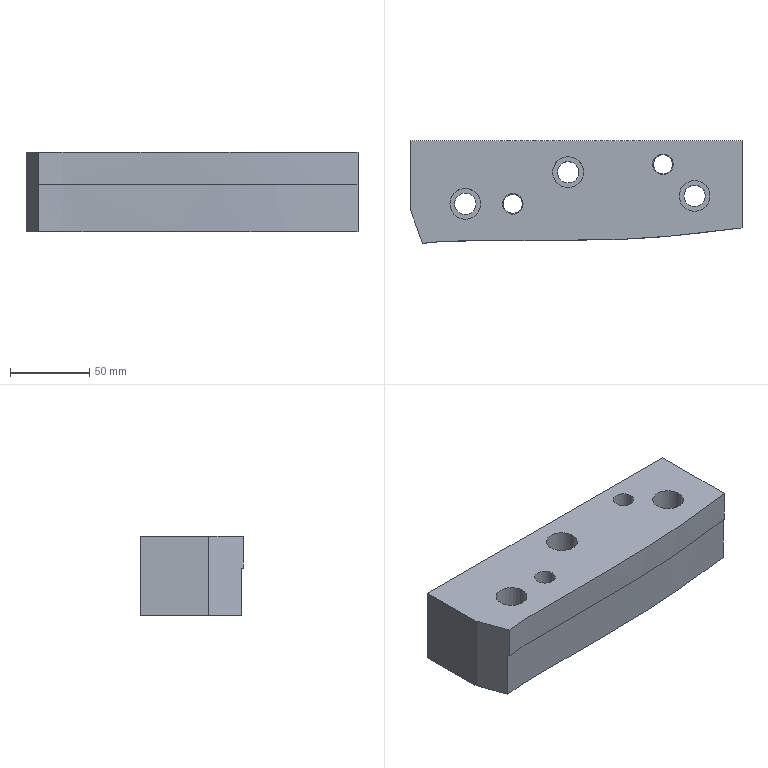Part | NX | features solid 2 | 1 solid | 24 faces | box 210 x 65.035 x 50 mm | volume 599667 mm3 | plane 12 | cylinder 10 | spline 2 | commonest cylinder face diameters 13.5 x3 19.5 x3 12 x2 13 x2
STEP:
#1=CARTESIAN_POINT('',(-107.046,-95.035,-20.));
#2=VERTEX_POINT('',#1);
#3=CARTESIAN_POINT('',(-107.046,-95.035,0.));
#4=VERTEX_POINT('',#3);
#5=CARTESIAN_POINT('',(-107.046,-95.035,-25.));
#6=DIRECTION('',(0.,0.,-1.));
#7=VECTOR('',#6,1000.);
#8=LINE('',#5,#7);
#9=EDGE_CURVE('',#2,#4,#8,.F.);
#10=ORIENTED_EDGE('',*,*,#9,.F.);
#11=CARTESIAN_POINT('',(95.,-85.269,-20.));
#12=VERTEX_POINT('',#11);
#13=CARTESIAN_POINT('',(-190.231,-121.49,-20.));
#14=CARTESIAN_POINT('',(-188.654,-121.152,-20.));
#15=CARTESIAN_POINT('',(-185.47,-120.627,-20.));
#16=CARTESIAN_POINT('',(-180.656,-120.141,-20.));
#17=CARTESIAN_POINT('',(-175.882,-119.326,-20.));
#18=CARTESIAN_POINT('',(-169.679,-117.528,-20.));
#19=CARTESIAN_POINT('',(-162.185,-114.539,-20.));
#20=CARTESIAN_POINT('',(-153.086,-111.254,-20.));
#21=CARTESIAN_POINT('',(-144.031,-107.845,-20.));
#22=CARTESIAN_POINT('',(-136.465,-105.061,-20.));
#23=CARTESIAN_POINT('',(-130.418,-102.814,-20.));
#24=CARTESIAN_POINT('',(-125.812,-101.329,-20.));
#25=CARTESIAN_POINT('',(-121.306,-99.566,-20.));
#26=CARTESIAN_POINT('',(-116.876,-97.626,-20.));
#27=CARTESIAN_POINT('',(-112.335,-95.923,-20.));
#28=CARTESIAN_POINT('',(-107.564,-95.05,-20.));
#29=CARTESIAN_POINT('',(-102.756,-94.525,-20.));
#30=CARTESIAN_POINT('',(-96.349,-93.771,-20.));
#31=CARTESIAN_POINT('',(-89.902,-93.468,-20.));
#32=CARTESIAN_POINT('',(-83.452,-93.448,-20.));
#33=CARTESIAN_POINT('',(-77.002,-93.469,-20.));
#34=CARTESIAN_POINT('',(-68.939,-93.411,-20.));
#35=CARTESIAN_POINT('',(-56.04,-93.3,-20.));
#36=CARTESIAN_POINT('',(-33.465,-93.184,-20.));
#37=CARTESIAN_POINT('',(-7.666,-93.074,-20.));
#38=CARTESIAN_POINT('',(14.907,-92.653,-20.));
#39=CARTESIAN_POINT('',(27.794,-92.068,-20.));
#40=CARTESIAN_POINT('',(40.668,-91.245,-20.));
#41=CARTESIAN_POINT('',(51.917,-90.291,-20.));
#42=CARTESIAN_POINT('',(61.528,-89.174,-20.));
#43=CARTESIAN_POINT('',(67.939,-88.466,-20.));
#44=CARTESIAN_POINT('',(79.125,-86.95,-20.));
#45=CARTESIAN_POINT('',(95.161,-85.253,-20.));
#46=CARTESIAN_POINT('',(114.404,-83.21,-20.));
#47=CARTESIAN_POINT('',(133.568,-80.524,-20.));
#48=CARTESIAN_POINT('',(152.734,-77.861,-20.));
#49=CARTESIAN_POINT('',(171.916,-75.326,-20.));
#50=CARTESIAN_POINT('',(191.055,-72.413,-20.));
#51=CARTESIAN_POINT('',(207.17,-71.468,-20.));
#52=CARTESIAN_POINT('',(219.951,-69.697,-20.));
#53=CARTESIAN_POINT('',(232.724,-67.899,-20.));
#54=CARTESIAN_POINT('',(248.708,-65.766,-20.));
#55=CARTESIAN_POINT('',(267.87,-63.074,-20.));
#56=CARTESIAN_POINT('',(287.038,-60.44,-20.));
#57=CARTESIAN_POINT('',(301.448,-58.682,-20.));
#58=CARTESIAN_POINT('',(310.976,-56.987,-20.));
#59=CARTESIAN_POINT('',(314.916,-56.135,-20.));
#60=CARTESIAN_POINT('',(318.052,-55.382,-20.));
#61=CARTESIAN_POINT('',(320.39,-54.76,-20.));
#62=CARTESIAN_POINT('',(322.686,-53.981,-20.));
#63=CARTESIAN_POINT('',(325.595,-52.578,-20.));
#64=CARTESIAN_POINT('',(328.769,-50.098,-20.));
#65=CARTESIAN_POINT('',(332.247,-46.69,-20.));
#66=CARTESIAN_POINT('',(335.795,-43.406,-20.));
#67=CARTESIAN_POINT('',(343.661,-37.758,-20.));
#68=CARTESIAN_POINT('',(355.164,-28.914,-20.));
#69=CARTESIAN_POINT('',(370.422,-17.018,-20.));
#70=CARTESIAN_POINT('',(383.264,-7.249,-20.));
#71=CARTESIAN_POINT('',(392.416,-0.6713,-20.));
#72=CARTESIAN_POINT('',(396.953,2.733,-20.));
#73=CARTESIAN_POINT('',(398.886,5.372,-20.));
#74=CARTESIAN_POINT('',(399.725,7.654,-20.));
#75=CARTESIAN_POINT('',(399.76,10.078,-20.));
#76=CARTESIAN_POINT('',(399.483,13.317,-20.));
#77=CARTESIAN_POINT('',(399.712,17.34,-20.));
#78=CARTESIAN_POINT('',(399.612,22.179,-20.));
#79=CARTESIAN_POINT('',(399.633,31.854,-20.));
#80=CARTESIAN_POINT('',(399.593,46.366,-20.));
#81=CARTESIAN_POINT('',(399.637,62.491,-20.));
#82=CARTESIAN_POINT('',(399.588,73.779,-20.));
#83=CARTESIAN_POINT('',(399.652,79.422,-20.));
#84=CARTESIAN_POINT('',(399.59,82.647,-20.));
#85=CARTESIAN_POINT('',(399.564,85.065,-20.));
#86=CARTESIAN_POINT('',(399.725,87.486,-20.));
#87=CARTESIAN_POINT('',(399.756,89.902,-20.));
#88=CARTESIAN_POINT('',(399.247,92.301,-20.));
#89=CARTESIAN_POINT('',(397.362,95.008,-20.));
#90=CARTESIAN_POINT('',(393.635,96.774,-20.));
#91=CARTESIAN_POINT('',(389.279,98.826,-20.));
#92=CARTESIAN_POINT('',(384.732,100.498,-20.));
#93=CARTESIAN_POINT('',(378.765,102.95,-20.));
#94=CARTESIAN_POINT('',(362.589,110.229,-20.));
#95=CARTESIAN_POINT('',(344.928,118.135,-20.));
#96=CARTESIAN_POINT('',(327.281,126.072,-20.));
#97=CARTESIAN_POINT('',(319.932,129.381,-20.));
#98=CARTESIAN_POINT('',(314.075,132.102,-20.));
#99=CARTESIAN_POINT('',(309.387,133.376,-20.));
#100=CARTESIAN_POINT('',(304.547,133.785,-20.));
#101=CARTESIAN_POINT('',(299.716,133.401,-20.));
#102=CARTESIAN_POINT('',(294.929,132.704,-20.));
#103=CARTESIAN_POINT('',(288.543,131.8,-20.));
#104=CARTESIAN_POINT('',(277.364,130.241,-20.));
#105=CARTESIAN_POINT('',(242.2,125.552,-20.));
#106=CARTESIAN_POINT('',(184.637,118.048,-20.));
#107=CARTESIAN_POINT('',(120.701,109.541,-20.));
#108=CARTESIAN_POINT('',(69.531,102.902,-20.));
#109=CARTESIAN_POINT('',(40.777,98.94,-20.));
#110=CARTESIAN_POINT('',(21.566,96.615,-20.));
#111=CARTESIAN_POINT('',(8.743,95.212,-20.));
#112=CARTESIAN_POINT('',(-7.301,93.575,-20.));
#113=CARTESIAN_POINT('',(-26.625,92.505,-20.));
#114=CARTESIAN_POINT('',(-45.971,92.017,-20.));
#115=CARTESIAN_POINT('',(-62.09,91.675,-20.));
#116=CARTESIAN_POINT('',(-74.987,91.256,-20.));
#117=CARTESIAN_POINT('',(-84.664,91.165,-20.));
#118=CARTESIAN_POINT('',(-94.319,91.781,-20.));
#119=CARTESIAN_POINT('',(-103.929,92.966,-20.));
#120=CARTESIAN_POINT('',(-113.495,94.403,-20.));
#121=CARTESIAN_POINT('',(-119.856,95.492,-20.));
#122=CARTESIAN_POINT('',(-122.997,96.222,-20.));
#123=B_SPLINE_CURVE_WITH_KNOTS('',3,(#13,#14,#15,#16,#17,#18,#19,#20,#21,#22,#23,#24,#25,#26,#27,#28,#29,#30,#31,#32,#33,#34,#35,#36,#37,#38,#39,#40,#41,#42,#43,#44,#45,#46,#47,#48,#49,#50,#51,#52,#53,#54,#55,#56,#57,#58,#59,#60,#61,#62,#63,#64,#65,#66,#67,#68,#69,#70,#71,#72,#73,#74,#75,#76,#77,#78,#79,#80,#81,#82,#83,#84,#85,#86,#87,#88,#89,#90,#91,#92,#93,#94,#95,#96,#97,#98,#99,#100,#101,#102,#103,#104,#105,#106,#107,#108,#109,#110,#111,#112,#113,#114,#115,#116,#117,#118,#119,#120,#121,#122),.UNSPECIFIED.,.F.,.F.,(4,1,1,1,1,1,1,1,1,1,1,1,1,1,1,1,1,1,1,1,1,1,1,1,1,1,1,1,1,1,1,1,1,1,1,1,1,1,1,1,1,1,1,1,1,1,1,1,1,1,1,1,1,1,1,1,1,1,1,1,1,1,1,1,1,1,1,1,1,1,1,1,1,1,1,1,1,1,1,1,1,1,1,1,1,1,1,1,1,1,1,1,1,1,1,1,1,1,1,1,1,1,1,1,1,1,1,4),(0.4704,0.4724,0.4745,0.4766,0.4786,0.4828,0.4869,0.491,0.4952,0.4972,0.4993,0.5014,0.5035,0.5055,0.5076,0.5097,0.5117,0.5159,0.5179,0.52,0.5241,0.5283,0.5366,0.5531,0.5614,0.5655,0.5697,0.5779,0.58,0.5821,0.5862,0.5945,0.6028,0.611,0.6193,0.6276,0.6359,0.6441,0.6483,0.6524,0.6607,0.669,0.6772,0.6855,0.6876,0.6897,0.6907,0.6917,0.6928,0.6938,0.6959,0.6979,0.7,0.7021,0.7103,0.7186,0.7269,0.731,0.7331,0.7341,0.7352,0.7362,0.7372,0.7393,0.7414,0.7435,0.7517,0.76,0.7641,0.7662,0.7672,0.7683,0.7693,0.7703,0.7714,0.7724,0.7745,0.7766,0.7786,0.7807,0.7848,0.8014,0.8055,0.8097,0.8117,0.8138,0.8159,0.8179,0.82,0.8221,0.8262,0.8345,0.8676,0.9007,0.9172,0.9338,0.9379,0.9421,0.9503,0.9586,0.9669,0.9752,0.9793,0.9834,0.9876,0.9917,0.9959,1.),.UNSPECIFIED.);
#124=EDGE_CURVE('',#2,#12,#123,.T.);
#125=ORIENTED_EDGE('',*,*,#124,.T.);
#126=CARTESIAN_POINT('',(95.,-85.269,0.));
#127=VERTEX_POINT('',#126);
#128=CARTESIAN_POINT('',(95.,-85.269,-10.));
#129=DIRECTION('',(0.,0.,-1.));
#130=VECTOR('',#129,1000.);
#131=LINE('',#128,#130);
#132=EDGE_CURVE('',#127,#12,#131,.T.);
#133=ORIENTED_EDGE('',*,*,#132,.F.);
#134=CARTESIAN_POINT('',(95.,-85.269,0.));
#135=CARTESIAN_POINT('',(90.809,-85.713,0.));
#136=CARTESIAN_POINT('',(82.426,-86.582,0.));
#137=CARTESIAN_POINT('',(69.877,-88.217,0.));
#138=CARTESIAN_POINT('',(57.316,-89.701,0.));
#139=CARTESIAN_POINT('',(40.542,-91.326,0.));
#140=CARTESIAN_POINT('',(19.52,-92.617,0.));
#141=CARTESIAN_POINT('',(-5.792,-93.02,0.));
#142=CARTESIAN_POINT('',(-31.119,-93.19,0.));
#143=CARTESIAN_POINT('',(-52.226,-93.263,0.));
#144=CARTESIAN_POINT('',(-69.108,-93.423,0.));
#145=CARTESIAN_POINT('',(-81.772,-93.467,0.));
#146=CARTESIAN_POINT('',(-92.328,-93.446,0.));
#147=CARTESIAN_POINT('',(-100.741,-94.276,0.));
#148=CARTESIAN_POINT('',(-104.946,-94.744,0.));
#149=CARTESIAN_POINT('',(-107.046,-95.035,0.));
#150=B_SPLINE_CURVE_WITH_KNOTS('',3,(#134,#135,#136,#137,#138,#139,#140,#141,#142,#143,#144,#145,#146,#147,#148,#149),.UNSPECIFIED.,.F.,.F.,(4,1,1,1,1,1,1,1,1,1,1,1,1,4),(0.,0.01264,0.02527,0.03791,0.05054,0.07582,0.1011,0.1264,0.1516,0.1643,0.1769,0.1895,0.1959,0.2022),.UNSPECIFIED.);
#151=EDGE_CURVE('',#127,#4,#150,.T.);
#152=ORIENTED_EDGE('',*,*,#151,.T.);
#153=EDGE_LOOP('',(#10,#125,#133,#152));
#154=FACE_BOUND('',#153,.T.);
#155=CARTESIAN_POINT('',(-107.046,-95.035,0.));
#156=CARTESIAN_POINT('',(-107.046,-95.035,-20.));
#157=CARTESIAN_POINT('',(-104.956,-94.746,0.));
#158=CARTESIAN_POINT('',(-104.956,-94.746,-20.));
#159=CARTESIAN_POINT('',(-100.763,-94.279,0.));
#160=CARTESIAN_POINT('',(-100.763,-94.279,-20.));
#161=CARTESIAN_POINT('',(-92.365,-93.447,0.));
#162=CARTESIAN_POINT('',(-92.365,-93.447,-20.));
#163=CARTESIAN_POINT('',(-81.808,-93.466,0.));
#164=CARTESIAN_POINT('',(-81.808,-93.466,-20.));
#165=CARTESIAN_POINT('',(-69.155,-93.424,0.));
#166=CARTESIAN_POINT('',(-69.155,-93.424,-20.));
#167=CARTESIAN_POINT('',(-52.28,-93.263,0.));
#168=CARTESIAN_POINT('',(-52.28,-93.263,-20.));
#169=CARTESIAN_POINT('',(-31.187,-93.19,0.));
#170=CARTESIAN_POINT('',(-31.187,-93.19,-20.));
#171=CARTESIAN_POINT('',(-5.876,-93.02,0.));
#172=CARTESIAN_POINT('',(-5.876,-93.02,-20.));
#173=CARTESIAN_POINT('',(19.435,-92.62,0.));
#174=CARTESIAN_POINT('',(19.435,-92.62,-20.));
#175=CARTESIAN_POINT('',(40.496,-91.329,0.));
#176=CARTESIAN_POINT('',(40.496,-91.329,-20.));
#177=CARTESIAN_POINT('',(57.293,-89.704,0.));
#178=CARTESIAN_POINT('',(57.293,-89.704,-20.));
#179=CARTESIAN_POINT('',(69.862,-88.219,0.));
#180=CARTESIAN_POINT('',(69.862,-88.219,-20.));
#181=CARTESIAN_POINT('',(82.412,-86.583,0.));
#182=CARTESIAN_POINT('',(82.412,-86.583,-20.));
#183=CARTESIAN_POINT('',(90.805,-85.714,0.));
#184=CARTESIAN_POINT('',(90.805,-85.714,-20.));
#185=CARTESIAN_POINT('',(95.,-85.269,0.));
#186=CARTESIAN_POINT('',(95.,-85.269,-20.));
#187=B_SPLINE_SURFACE_WITH_KNOTS('',3,1,((#155,#156),(#157,#158),(#159,#160),(#161,#162),(#163,#164),(#165,#166),(#167,#168),(#169,#170),(#171,#172),(#173,#174),(#175,#176),(#177,#178),(#179,#180),(#181,#182),(#183,#184),(#185,#186)),.SURF_OF_LINEAR_EXTRUSION.,.F.,.F.,.F.,(4,1,1,1,1,1,1,1,1,1,1,1,1,4),(2,2),(0.5078,0.5105,0.5132,0.5186,0.5241,0.5295,0.5403,0.5511,0.5619,0.5728,0.5782,0.5836,0.589,0.5944),(0.,1.),.UNSPECIFIED.);
#188=ADVANCED_FACE('',(#154),#187,.F.);
#189=CARTESIAN_POINT('',(95.,-84.264,-20.));
#190=VERTEX_POINT('',#189);
#191=CARTESIAN_POINT('',(95.,83.097,-20.));
#192=DIRECTION('',(0.,-1.,0.));
#193=VECTOR('',#192,1000.);
#194=LINE('',#191,#193);
#195=EDGE_CURVE('',#190,#12,#194,.T.);
#196=ORIENTED_EDGE('',*,*,#195,.F.);
#197=CARTESIAN_POINT('',(95.,-84.264,-50.));
#198=VERTEX_POINT('',#197);
#199=CARTESIAN_POINT('',(95.,-84.264,-60.));
#200=DIRECTION('',(0.,0.,-1.));
#201=VECTOR('',#200,1000.);
#202=LINE('',#199,#201);
#203=EDGE_CURVE('',#198,#190,#202,.F.);
#204=ORIENTED_EDGE('',*,*,#203,.F.);
#205=CARTESIAN_POINT('',(95.,-30.,-50.));
#206=VERTEX_POINT('',#205);
#207=CARTESIAN_POINT('',(95.,35.09,-50.));
#208=DIRECTION('',(0.,1.,0.));
#209=VECTOR('',#208,1000.);
#210=LINE('',#207,#209);
#211=EDGE_CURVE('',#198,#206,#210,.T.);
#212=ORIENTED_EDGE('',*,*,#211,.T.);
#213=CARTESIAN_POINT('',(95.,-30.,0.));
#214=VERTEX_POINT('',#213);
#215=CARTESIAN_POINT('',(95.,-30.,0.));
#216=DIRECTION('',(0.,0.,-1.));
#217=VECTOR('',#216,1000.);
#218=LINE('',#215,#217);
#219=EDGE_CURVE('',#214,#206,#218,.T.);
#220=ORIENTED_EDGE('',*,*,#219,.F.);
#221=CARTESIAN_POINT('',(95.,-222.,0.));
#222=DIRECTION('',(0.,-1.,0.));
#223=VECTOR('',#222,1000.);
#224=LINE('',#221,#223);
#225=EDGE_CURVE('',#214,#127,#224,.T.);
#226=ORIENTED_EDGE('',*,*,#225,.T.);
#227=ORIENTED_EDGE('',*,*,#132,.T.);
#228=EDGE_LOOP('',(#196,#204,#212,#220,#226,#227));
#229=FACE_BOUND('',#228,.T.);
#230=CARTESIAN_POINT('',(95.,83.097,-25.));
#231=DIRECTION('',(1.,0.,0.));
#232=DIRECTION('',(0.,0.,-1.));
#233=AXIS2_PLACEMENT_3D('',#230,#231,#232);
#234=PLANE('',#233);
#235=ADVANCED_FACE('',(#229),#234,.T.);
#236=CARTESIAN_POINT('',(-115.,-73.182,-50.));
#237=VERTEX_POINT('',#236);
#238=CARTESIAN_POINT('',(-115.,-30.,-50.));
#239=VERTEX_POINT('',#238);
#240=CARTESIAN_POINT('',(-115.,35.09,-50.));
#241=DIRECTION('',(0.,1.,0.));
#242=VECTOR('',#241,1000.);
#243=LINE('',#240,#242);
#244=EDGE_CURVE('',#237,#239,#243,.T.);
#245=ORIENTED_EDGE('',*,*,#244,.F.);
#246=CARTESIAN_POINT('',(-115.,-73.182,0.));
#247=VERTEX_POINT('',#246);
#248=CARTESIAN_POINT('',(-115.,-73.182,0.));
#249=DIRECTION('',(0.,0.,1.));
#250=VECTOR('',#249,1000.);
#251=LINE('',#248,#250);
#252=EDGE_CURVE('',#237,#247,#251,.T.);
#253=ORIENTED_EDGE('',*,*,#252,.T.);
#254=CARTESIAN_POINT('',(-115.,-30.,0.));
#255=VERTEX_POINT('',#254);
#256=CARTESIAN_POINT('',(-115.,-222.,0.));
#257=DIRECTION('',(0.,-1.,0.));
#258=VECTOR('',#257,1000.);
#259=LINE('',#256,#258);
#260=EDGE_CURVE('',#255,#247,#259,.T.);
#261=ORIENTED_EDGE('',*,*,#260,.F.);
#262=CARTESIAN_POINT('',(-115.,-30.,0.));
#263=DIRECTION('',(0.,0.,1.));
#264=VECTOR('',#263,1000.);
#265=LINE('',#262,#264);
#266=EDGE_CURVE('',#239,#255,#265,.T.);
#267=ORIENTED_EDGE('',*,*,#266,.F.);
#268=EDGE_LOOP('',(#245,#253,#261,#267));
#269=FACE_BOUND('',#268,.T.);
#270=CARTESIAN_POINT('',(-115.,30.,0.));
#271=DIRECTION('',(1.,0.,0.));
#272=DIRECTION('',(0.,0.,-1.));
#273=AXIS2_PLACEMENT_3D('',#270,#271,#272);
#274=PLANE('',#273);
#275=ADVANCED_FACE('',(#269),#274,.F.);
#276=CARTESIAN_POINT('',(-56.5,-70.,0.));
#277=VERTEX_POINT('',#276);
#278=CARTESIAN_POINT('',(-50.,-70.,0.));
#279=DIRECTION('',(0.,0.,-1.));
#280=DIRECTION('',(-1.,0.,0.));
#281=AXIS2_PLACEMENT_3D('',#278,#279,#280);
#282=CIRCLE('',#281,6.5);
#283=EDGE_CURVE('',#277,#277,#282,.T.);
#284=ORIENTED_EDGE('',*,*,#283,.T.);
#285=EDGE_LOOP('',(#284));
#286=FACE_BOUND('',#285,.T.);
#287=CARTESIAN_POINT('',(38.5,-45.,0.));
#288=VERTEX_POINT('',#287);
#289=CARTESIAN_POINT('',(45.,-45.,0.));
#290=DIRECTION('',(0.,0.,-1.));
#291=DIRECTION('',(-1.,0.,0.));
#292=AXIS2_PLACEMENT_3D('',#289,#290,#291);
#293=CIRCLE('',#292,6.5);
#294=EDGE_CURVE('',#288,#288,#293,.T.);
#295=ORIENTED_EDGE('',*,*,#294,.T.);
#296=EDGE_LOOP('',(#295));
#297=FACE_BOUND('',#296,.T.);
#298=CARTESIAN_POINT('',(-89.75,-70.,0.));
#299=VERTEX_POINT('',#298);
#300=CARTESIAN_POINT('',(-80.,-70.,0.));
#301=DIRECTION('',(0.,0.,-1.));
#302=DIRECTION('',(-1.,0.,0.));
#303=AXIS2_PLACEMENT_3D('',#300,#301,#302);
#304=CIRCLE('',#303,9.75);
#305=EDGE_CURVE('',#299,#299,#304,.T.);
#306=ORIENTED_EDGE('',*,*,#305,.T.);
#307=EDGE_LOOP('',(#306));
#308=FACE_BOUND('',#307,.T.);
#309=CARTESIAN_POINT('',(-24.75,-50.,0.));
#310=VERTEX_POINT('',#309);
#311=CARTESIAN_POINT('',(-15.,-50.,0.));
#312=DIRECTION('',(0.,0.,-1.));
#313=DIRECTION('',(-1.,0.,0.));
#314=AXIS2_PLACEMENT_3D('',#311,#312,#313);
#315=CIRCLE('',#314,9.75);
#316=EDGE_CURVE('',#310,#310,#315,.T.);
#317=ORIENTED_EDGE('',*,*,#316,.T.);
#318=EDGE_LOOP('',(#317));
#319=FACE_BOUND('',#318,.T.);
#320=CARTESIAN_POINT('',(55.25,-65.,0.));
#321=VERTEX_POINT('',#320);
#322=CARTESIAN_POINT('',(65.,-65.,0.));
#323=DIRECTION('',(0.,0.,-1.));
#324=DIRECTION('',(-1.,0.,0.));
#325=AXIS2_PLACEMENT_3D('',#322,#323,#324);
#326=CIRCLE('',#325,9.75);
#327=EDGE_CURVE('',#321,#321,#326,.T.);
#328=ORIENTED_EDGE('',*,*,#327,.T.);
#329=EDGE_LOOP('',(#328));
#330=FACE_BOUND('',#329,.T.);
#331=ORIENTED_EDGE('',*,*,#260,.T.);
#332=CARTESIAN_POINT('',(-108.743,-90.374,0.));
#333=DIRECTION('',(0.342,-0.9397,0.));
#334=VECTOR('',#333,1000.);
#335=LINE('',#332,#334);
#336=EDGE_CURVE('',#247,#4,#335,.T.);
#337=ORIENTED_EDGE('',*,*,#336,.T.);
#338=ORIENTED_EDGE('',*,*,#151,.F.);
#339=ORIENTED_EDGE('',*,*,#225,.F.);
#340=CARTESIAN_POINT('',(-470.381,-30.,0.));
#341=DIRECTION('',(1.,0.,0.));
#342=VECTOR('',#341,1000.);
#343=LINE('',#340,#342);
#344=EDGE_CURVE('',#255,#214,#343,.T.);
#345=ORIENTED_EDGE('',*,*,#344,.F.);
#346=EDGE_LOOP('',(#331,#337,#338,#339,#345));
#347=FACE_BOUND('',#346,.T.);
#348=CARTESIAN_POINT('',(-470.381,-222.,0.));
#349=DIRECTION('',(0.,0.,-1.));
#350=DIRECTION('',(-1.,0.,0.));
#351=AXIS2_PLACEMENT_3D('',#348,#349,#350);
#352=PLANE('',#351);
#353=ADVANCED_FACE('',(#286,#297,#308,#319,#330,#347),#352,.F.);
#354=ORIENTED_EDGE('',*,*,#344,.T.);
#355=ORIENTED_EDGE('',*,*,#219,.T.);
#356=CARTESIAN_POINT('',(-415.478,-30.,-50.));
#357=DIRECTION('',(-1.,0.,0.));
#358=VECTOR('',#357,1000.);
#359=LINE('',#356,#358);
#360=EDGE_CURVE('',#206,#239,#359,.T.);
#361=ORIENTED_EDGE('',*,*,#360,.T.);
#362=ORIENTED_EDGE('',*,*,#266,.T.);
#363=EDGE_LOOP('',(#354,#355,#361,#362));
#364=FACE_BOUND('',#363,.T.);
#365=CARTESIAN_POINT('',(190.,-30.,0.));
#366=DIRECTION('',(0.,1.,0.));
#367=DIRECTION('',(0.,0.,1.));
#368=AXIS2_PLACEMENT_3D('',#365,#366,#367);
#369=PLANE('',#368);
#370=ADVANCED_FACE('',(#364),#369,.T.);
#371=CARTESIAN_POINT('',(-44.,-70.,-50.));
#372=VERTEX_POINT('',#371);
#373=CARTESIAN_POINT('',(-50.,-70.,-50.));
#374=DIRECTION('',(0.,0.,1.));
#375=DIRECTION('',(1.,0.,0.));
#376=AXIS2_PLACEMENT_3D('',#373,#374,#375);
#377=CIRCLE('',#376,6.);
#378=EDGE_CURVE('',#372,#372,#377,.T.);
#379=ORIENTED_EDGE('',*,*,#378,.T.);
#380=EDGE_LOOP('',(#379));
#381=FACE_BOUND('',#380,.T.);
#382=CARTESIAN_POINT('',(51.,-45.,-50.));
#383=VERTEX_POINT('',#382);
#384=CARTESIAN_POINT('',(45.,-45.,-50.));
#385=DIRECTION('',(0.,0.,1.));
#386=DIRECTION('',(1.,0.,0.));
#387=AXIS2_PLACEMENT_3D('',#384,#385,#386);
#388=CIRCLE('',#387,6.);
#389=EDGE_CURVE('',#383,#383,#388,.T.);
#390=ORIENTED_EDGE('',*,*,#389,.T.);
#391=EDGE_LOOP('',(#390));
#392=FACE_BOUND('',#391,.T.);
#393=CARTESIAN_POINT('',(-73.25,-70.,-50.));
#394=VERTEX_POINT('',#393);
#395=CARTESIAN_POINT('',(-80.,-70.,-50.));
#396=DIRECTION('',(0.,0.,1.));
#397=DIRECTION('',(1.,0.,0.));
#398=AXIS2_PLACEMENT_3D('',#395,#396,#397);
#399=CIRCLE('',#398,6.75);
#400=EDGE_CURVE('',#394,#394,#399,.T.);
#401=ORIENTED_EDGE('',*,*,#400,.T.);
#402=EDGE_LOOP('',(#401));
#403=FACE_BOUND('',#402,.T.);
#404=CARTESIAN_POINT('',(-8.25,-50.,-50.));
#405=VERTEX_POINT('',#404);
#406=CARTESIAN_POINT('',(-15.,-50.,-50.));
#407=DIRECTION('',(0.,0.,1.));
#408=DIRECTION('',(1.,0.,0.));
#409=AXIS2_PLACEMENT_3D('',#406,#407,#408);
#410=CIRCLE('',#409,6.75);
#411=EDGE_CURVE('',#405,#405,#410,.T.);
#412=ORIENTED_EDGE('',*,*,#411,.T.);
#413=EDGE_LOOP('',(#412));
#414=FACE_BOUND('',#413,.T.);
#415=CARTESIAN_POINT('',(71.75,-65.,-50.));
#416=VERTEX_POINT('',#415);
#417=CARTESIAN_POINT('',(65.,-65.,-50.));
#418=DIRECTION('',(0.,0.,1.));
#419=DIRECTION('',(1.,0.,0.));
#420=AXIS2_PLACEMENT_3D('',#417,#418,#419);
#421=CIRCLE('',#420,6.75);
#422=EDGE_CURVE('',#416,#416,#421,.T.);
#423=ORIENTED_EDGE('',*,*,#422,.T.);
#424=EDGE_LOOP('',(#423));
#425=FACE_BOUND('',#424,.T.);
#426=ORIENTED_EDGE('',*,*,#211,.F.);
#427=CARTESIAN_POINT('',(-107.396,-94.075,-50.));
#428=VERTEX_POINT('',#427);
#429=CARTESIAN_POINT('',(95.,-84.264,-50.));
#430=CARTESIAN_POINT('',(90.802,-84.709,-50.));
#431=CARTESIAN_POINT('',(82.405,-85.578,-50.));
#432=CARTESIAN_POINT('',(69.834,-87.213,-50.));
#433=CARTESIAN_POINT('',(57.253,-88.703,-50.));
#434=CARTESIAN_POINT('',(40.45,-90.33,-50.));
#435=CARTESIAN_POINT('',(19.392,-91.622,-50.));
#436=CARTESIAN_POINT('',(-5.964,-92.021,-50.));
#437=CARTESIAN_POINT('',(-31.334,-92.191,-50.));
#438=CARTESIAN_POINT('',(-52.477,-92.263,-50.));
#439=CARTESIAN_POINT('',(-69.388,-92.427,-50.));
#440=CARTESIAN_POINT('',(-82.074,-92.461,-50.));
#441=CARTESIAN_POINT('',(-92.647,-92.457,-50.));
#442=CARTESIAN_POINT('',(-101.077,-93.311,-50.));
#443=CARTESIAN_POINT('',(-105.291,-93.777,-50.));
#444=CARTESIAN_POINT('',(-107.396,-94.075,-50.));
#445=B_SPLINE_CURVE_WITH_KNOTS('',3,(#429,#430,#431,#432,#433,#434,#435,#436,#437,#438,#439,#440,#441,#442,#443,#444),.UNSPECIFIED.,.F.,.F.,(4,1,1,1,1,1,1,1,1,1,1,1,1,4),(0.,0.01266,0.02532,0.03797,0.05063,0.07595,0.1013,0.1266,0.1519,0.1645,0.1772,0.1899,0.1962,0.2025),.UNSPECIFIED.);
#446=EDGE_CURVE('',#198,#428,#445,.T.);
#447=ORIENTED_EDGE('',*,*,#446,.T.);
#448=CARTESIAN_POINT('',(-184.947,118.996,-50.));
#449=DIRECTION('',(-0.342,0.9397,0.));
#450=VECTOR('',#449,1000.);
#451=LINE('',#448,#450);
#452=EDGE_CURVE('',#428,#237,#451,.T.);
#453=ORIENTED_EDGE('',*,*,#452,.T.);
#454=ORIENTED_EDGE('',*,*,#244,.T.);
#455=ORIENTED_EDGE('',*,*,#360,.F.);
#456=EDGE_LOOP('',(#426,#447,#453,#454,#455));
#457=FACE_BOUND('',#456,.T.);
#458=CARTESIAN_POINT('',(-415.478,35.09,-50.));
#459=DIRECTION('',(0.,0.,1.));
#460=DIRECTION('',(1.,0.,0.));
#461=AXIS2_PLACEMENT_3D('',#458,#459,#460);
#462=PLANE('',#461);
#463=ADVANCED_FACE('',(#381,#392,#403,#414,#425,#457),#462,.F.);
#464=CARTESIAN_POINT('',(58.25,-65.,-15.));
#465=VERTEX_POINT('',#464);
#466=CARTESIAN_POINT('',(65.,-65.,-15.));
#467=DIRECTION('',(0.,0.,-1.));
#468=DIRECTION('',(-1.,0.,0.));
#469=AXIS2_PLACEMENT_3D('',#466,#467,#468);
#470=CIRCLE('',#469,6.75);
#471=EDGE_CURVE('',#465,#465,#470,.T.);
#472=ORIENTED_EDGE('',*,*,#471,.F.);
#473=EDGE_LOOP('',(#472));
#474=FACE_BOUND('',#473,.T.);
#475=ORIENTED_EDGE('',*,*,#422,.F.);
#476=EDGE_LOOP('',(#475));
#477=FACE_BOUND('',#476,.T.);
#478=CARTESIAN_POINT('',(65.,-65.,-100.));
#479=DIRECTION('',(0.,0.,-1.));
#480=DIRECTION('',(-1.,0.,0.));
#481=AXIS2_PLACEMENT_3D('',#478,#479,#480);
#482=CYLINDRICAL_SURFACE('',#481,6.75);
#483=ADVANCED_FACE('',(#474,#477),#482,.F.);
#484=ORIENTED_EDGE('',*,*,#471,.T.);
#485=EDGE_LOOP('',(#484));
#486=FACE_BOUND('',#485,.T.);
#487=CARTESIAN_POINT('',(55.25,-65.,-15.));
#488=VERTEX_POINT('',#487);
#489=CARTESIAN_POINT('',(65.,-65.,-15.));
#490=DIRECTION('',(0.,0.,-1.));
#491=DIRECTION('',(-1.,0.,0.));
#492=AXIS2_PLACEMENT_3D('',#489,#490,#491);
#493=CIRCLE('',#492,9.75);
#494=EDGE_CURVE('',#488,#488,#493,.T.);
#495=ORIENTED_EDGE('',*,*,#494,.F.);
#496=EDGE_LOOP('',(#495));
#497=FACE_BOUND('',#496,.T.);
#498=CARTESIAN_POINT('',(65.,-65.,-15.));
#499=DIRECTION('',(0.,0.,-1.));
#500=DIRECTION('',(-1.,0.,0.));
#501=AXIS2_PLACEMENT_3D('',#498,#499,#500);
#502=PLANE('',#501);
#503=ADVANCED_FACE('',(#486,#497),#502,.F.);
#504=ORIENTED_EDGE('',*,*,#494,.T.);
#505=EDGE_LOOP('',(#504));
#506=FACE_BOUND('',#505,.T.);
#507=ORIENTED_EDGE('',*,*,#327,.F.);
#508=EDGE_LOOP('',(#507));
#509=FACE_BOUND('',#508,.T.);
#510=CARTESIAN_POINT('',(65.,-65.,0.));
#511=DIRECTION('',(0.,0.,-1.));
#512=DIRECTION('',(-1.,0.,0.));
#513=AXIS2_PLACEMENT_3D('',#510,#511,#512);
#514=CYLINDRICAL_SURFACE('',#513,9.75);
#515=ADVANCED_FACE('',(#506,#509),#514,.F.);
#516=CARTESIAN_POINT('',(-21.75,-50.,-15.));
#517=VERTEX_POINT('',#516);
#518=CARTESIAN_POINT('',(-15.,-50.,-15.));
#519=DIRECTION('',(0.,0.,-1.));
#520=DIRECTION('',(-1.,0.,0.));
#521=AXIS2_PLACEMENT_3D('',#518,#519,#520);
#522=CIRCLE('',#521,6.75);
#523=EDGE_CURVE('',#517,#517,#522,.T.);
#524=ORIENTED_EDGE('',*,*,#523,.F.);
#525=EDGE_LOOP('',(#524));
#526=FACE_BOUND('',#525,.T.);
#527=ORIENTED_EDGE('',*,*,#411,.F.);
#528=EDGE_LOOP('',(#527));
#529=FACE_BOUND('',#528,.T.);
#530=CARTESIAN_POINT('',(-15.,-50.,-100.));
#531=DIRECTION('',(0.,0.,-1.));
#532=DIRECTION('',(-1.,0.,0.));
#533=AXIS2_PLACEMENT_3D('',#530,#531,#532);
#534=CYLINDRICAL_SURFACE('',#533,6.75);
#535=ADVANCED_FACE('',(#526,#529),#534,.F.);
#536=ORIENTED_EDGE('',*,*,#523,.T.);
#537=EDGE_LOOP('',(#536));
#538=FACE_BOUND('',#537,.T.);
#539=CARTESIAN_POINT('',(-24.75,-50.,-15.));
#540=VERTEX_POINT('',#539);
#541=CARTESIAN_POINT('',(-15.,-50.,-15.));
#542=DIRECTION('',(0.,0.,-1.));
#543=DIRECTION('',(-1.,0.,0.));
#544=AXIS2_PLACEMENT_3D('',#541,#542,#543);
#545=CIRCLE('',#544,9.75);
#546=EDGE_CURVE('',#540,#540,#545,.T.);
#547=ORIENTED_EDGE('',*,*,#546,.F.);
#548=EDGE_LOOP('',(#547));
#549=FACE_BOUND('',#548,.T.);
#550=CARTESIAN_POINT('',(-15.,-55.,-15.));
#551=DIRECTION('',(0.,0.,-1.));
#552=DIRECTION('',(-1.,0.,0.));
#553=AXIS2_PLACEMENT_3D('',#550,#551,#552);
#554=PLANE('',#553);
#555=ADVANCED_FACE('',(#538,#549),#554,.F.);
#556=ORIENTED_EDGE('',*,*,#546,.T.);
#557=EDGE_LOOP('',(#556));
#558=FACE_BOUND('',#557,.T.);
#559=ORIENTED_EDGE('',*,*,#316,.F.);
#560=EDGE_LOOP('',(#559));
#561=FACE_BOUND('',#560,.T.);
#562=CARTESIAN_POINT('',(-15.,-50.,0.));
#563=DIRECTION('',(0.,0.,-1.));
#564=DIRECTION('',(-1.,0.,0.));
#565=AXIS2_PLACEMENT_3D('',#562,#563,#564);
#566=CYLINDRICAL_SURFACE('',#565,9.75);
#567=ADVANCED_FACE('',(#558,#561),#566,.F.);
#568=CARTESIAN_POINT('',(-86.75,-70.,-15.));
#569=VERTEX_POINT('',#568);
#570=CARTESIAN_POINT('',(-80.,-70.,-15.));
#571=DIRECTION('',(0.,0.,-1.));
#572=DIRECTION('',(-1.,0.,0.));
#573=AXIS2_PLACEMENT_3D('',#570,#571,#572);
#574=CIRCLE('',#573,6.75);
#575=EDGE_CURVE('',#569,#569,#574,.T.);
#576=ORIENTED_EDGE('',*,*,#575,.F.);
#577=EDGE_LOOP('',(#576));
#578=FACE_BOUND('',#577,.T.);
#579=ORIENTED_EDGE('',*,*,#400,.F.);
#580=EDGE_LOOP('',(#579));
#581=FACE_BOUND('',#580,.T.);
#582=CARTESIAN_POINT('',(-80.,-70.,-100.));
#583=DIRECTION('',(0.,0.,-1.));
#584=DIRECTION('',(-1.,0.,0.));
#585=AXIS2_PLACEMENT_3D('',#582,#583,#584);
#586=CYLINDRICAL_SURFACE('',#585,6.75);
#587=ADVANCED_FACE('',(#578,#581),#586,.F.);
#588=ORIENTED_EDGE('',*,*,#575,.T.);
#589=EDGE_LOOP('',(#588));
#590=FACE_BOUND('',#589,.T.);
#591=CARTESIAN_POINT('',(-89.75,-70.,-15.));
#592=VERTEX_POINT('',#591);
#593=CARTESIAN_POINT('',(-80.,-70.,-15.));
#594=DIRECTION('',(0.,0.,-1.));
#595=DIRECTION('',(-1.,0.,0.));
#596=AXIS2_PLACEMENT_3D('',#593,#594,#595);
#597=CIRCLE('',#596,9.75);
#598=EDGE_CURVE('',#592,#592,#597,.T.);
#599=ORIENTED_EDGE('',*,*,#598,.F.);
#600=EDGE_LOOP('',(#599));
#601=FACE_BOUND('',#600,.T.);
#602=CARTESIAN_POINT('',(-80.,-75.,-15.));
#603=DIRECTION('',(0.,0.,-1.));
#604=DIRECTION('',(-1.,0.,0.));
#605=AXIS2_PLACEMENT_3D('',#602,#603,#604);
#606=PLANE('',#605);
#607=ADVANCED_FACE('',(#590,#601),#606,.F.);
#608=ORIENTED_EDGE('',*,*,#598,.T.);
#609=EDGE_LOOP('',(#608));
#610=FACE_BOUND('',#609,.T.);
#611=ORIENTED_EDGE('',*,*,#305,.F.);
#612=EDGE_LOOP('',(#611));
#613=FACE_BOUND('',#612,.T.);
#614=CARTESIAN_POINT('',(-80.,-70.,0.));
#615=DIRECTION('',(0.,0.,-1.));
#616=DIRECTION('',(-1.,0.,0.));
#617=AXIS2_PLACEMENT_3D('',#614,#615,#616);
#618=CYLINDRICAL_SURFACE('',#617,9.75);
#619=ADVANCED_FACE('',(#610,#613),#618,.F.);
#620=CARTESIAN_POINT('',(39.,-45.,-20.));
#621=VERTEX_POINT('',#620);
#622=CARTESIAN_POINT('',(45.,-45.,-20.));
#623=DIRECTION('',(0.,0.,-1.));
#624=DIRECTION('',(-1.,0.,0.));
#625=AXIS2_PLACEMENT_3D('',#622,#623,#624);
#626=CIRCLE('',#625,6.);
#627=EDGE_CURVE('',#621,#621,#626,.T.);
#628=ORIENTED_EDGE('',*,*,#627,.F.);
#629=EDGE_LOOP('',(#628));
#630=FACE_BOUND('',#629,.T.);
#631=ORIENTED_EDGE('',*,*,#389,.F.);
#632=EDGE_LOOP('',(#631));
#633=FACE_BOUND('',#632,.T.);
#634=CARTESIAN_POINT('',(45.,-45.,-100.));
#635=DIRECTION('',(0.,0.,-1.));
#636=DIRECTION('',(-1.,0.,0.));
#637=AXIS2_PLACEMENT_3D('',#634,#635,#636);
#638=CYLINDRICAL_SURFACE('',#637,6.);
#639=ADVANCED_FACE('',(#630,#633),#638,.F.);
#640=ORIENTED_EDGE('',*,*,#627,.T.);
#641=EDGE_LOOP('',(#640));
#642=FACE_BOUND('',#641,.T.);
#643=CARTESIAN_POINT('',(38.5,-45.,-20.));
#644=VERTEX_POINT('',#643);
#645=CARTESIAN_POINT('',(45.,-45.,-20.));
#646=DIRECTION('',(0.,0.,-1.));
#647=DIRECTION('',(-1.,0.,0.));
#648=AXIS2_PLACEMENT_3D('',#645,#646,#647);
#649=CIRCLE('',#648,6.5);
#650=EDGE_CURVE('',#644,#644,#649,.T.);
#651=ORIENTED_EDGE('',*,*,#650,.F.);
#652=EDGE_LOOP('',(#651));
#653=FACE_BOUND('',#652,.T.);
#654=CARTESIAN_POINT('',(50.,-45.,-20.));
#655=DIRECTION('',(0.,0.,-1.));
#656=DIRECTION('',(-1.,0.,0.));
#657=AXIS2_PLACEMENT_3D('',#654,#655,#656);
#658=PLANE('',#657);
#659=ADVANCED_FACE('',(#642,#653),#658,.F.);
#660=ORIENTED_EDGE('',*,*,#650,.T.);
#661=EDGE_LOOP('',(#660));
#662=FACE_BOUND('',#661,.T.);
#663=ORIENTED_EDGE('',*,*,#294,.F.);
#664=EDGE_LOOP('',(#663));
#665=FACE_BOUND('',#664,.T.);
#666=CARTESIAN_POINT('',(45.,-45.,0.));
#667=DIRECTION('',(0.,0.,-1.));
#668=DIRECTION('',(-1.,0.,0.));
#669=AXIS2_PLACEMENT_3D('',#666,#667,#668);
#670=CYLINDRICAL_SURFACE('',#669,6.5);
#671=ADVANCED_FACE('',(#662,#665),#670,.F.);
#672=CARTESIAN_POINT('',(-56.,-70.,-20.));
#673=VERTEX_POINT('',#672);
#674=CARTESIAN_POINT('',(-50.,-70.,-20.));
#675=DIRECTION('',(0.,0.,-1.));
#676=DIRECTION('',(-1.,0.,0.));
#677=AXIS2_PLACEMENT_3D('',#674,#675,#676);
#678=CIRCLE('',#677,6.);
#679=EDGE_CURVE('',#673,#673,#678,.T.);
#680=ORIENTED_EDGE('',*,*,#679,.F.);
#681=EDGE_LOOP('',(#680));
#682=FACE_BOUND('',#681,.T.);
#683=ORIENTED_EDGE('',*,*,#378,.F.);
#684=EDGE_LOOP('',(#683));
#685=FACE_BOUND('',#684,.T.);
#686=CARTESIAN_POINT('',(-50.,-70.,-100.));
#687=DIRECTION('',(0.,0.,-1.));
#688=DIRECTION('',(-1.,0.,0.));
#689=AXIS2_PLACEMENT_3D('',#686,#687,#688);
#690=CYLINDRICAL_SURFACE('',#689,6.);
#691=ADVANCED_FACE('',(#682,#685),#690,.F.);
#692=ORIENTED_EDGE('',*,*,#679,.T.);
#693=EDGE_LOOP('',(#692));
#694=FACE_BOUND('',#693,.T.);
#695=CARTESIAN_POINT('',(-56.5,-70.,-20.));
#696=VERTEX_POINT('',#695);
#697=CARTESIAN_POINT('',(-50.,-70.,-20.));
#698=DIRECTION('',(0.,0.,-1.));
#699=DIRECTION('',(-1.,0.,0.));
#700=AXIS2_PLACEMENT_3D('',#697,#698,#699);
#701=CIRCLE('',#700,6.5);
#702=EDGE_CURVE('',#696,#696,#701,.T.);
#703=ORIENTED_EDGE('',*,*,#702,.F.);
#704=EDGE_LOOP('',(#703));
#705=FACE_BOUND('',#704,.T.);
#706=CARTESIAN_POINT('',(-50.,-70.,-20.));
#707=DIRECTION('',(0.,0.,-1.));
#708=DIRECTION('',(-1.,0.,0.));
#709=AXIS2_PLACEMENT_3D('',#706,#707,#708);
#710=PLANE('',#709);
#711=ADVANCED_FACE('',(#694,#705),#710,.F.);
#712=ORIENTED_EDGE('',*,*,#702,.T.);
#713=EDGE_LOOP('',(#712));
#714=FACE_BOUND('',#713,.T.);
#715=ORIENTED_EDGE('',*,*,#283,.F.);
#716=EDGE_LOOP('',(#715));
#717=FACE_BOUND('',#716,.T.);
#718=CARTESIAN_POINT('',(-50.,-70.,0.));
#719=DIRECTION('',(0.,0.,-1.));
#720=DIRECTION('',(-1.,0.,0.));
#721=AXIS2_PLACEMENT_3D('',#718,#719,#720);
#722=CYLINDRICAL_SURFACE('',#721,6.5);
#723=ADVANCED_FACE('',(#714,#717),#722,.F.);
#724=CARTESIAN_POINT('',(-107.396,-94.075,-20.));
#725=VERTEX_POINT('',#724);
#726=CARTESIAN_POINT('',(-107.396,-94.075,-60.));
#727=DIRECTION('',(0.,0.,-1.));
#728=VECTOR('',#727,1000.);
#729=LINE('',#726,#728);
#730=EDGE_CURVE('',#428,#725,#729,.F.);
#731=ORIENTED_EDGE('',*,*,#730,.T.);
#732=CARTESIAN_POINT('',(-123.265,-50.473,-20.));
#733=DIRECTION('',(0.342,-0.9397,0.));
#734=VECTOR('',#733,1000.);
#735=LINE('',#732,#734);
#736=EDGE_CURVE('',#725,#2,#735,.T.);
#737=ORIENTED_EDGE('',*,*,#736,.T.);
#738=ORIENTED_EDGE('',*,*,#9,.T.);
#739=ORIENTED_EDGE('',*,*,#336,.F.);
#740=ORIENTED_EDGE('',*,*,#252,.F.);
#741=ORIENTED_EDGE('',*,*,#452,.F.);
#742=EDGE_LOOP('',(#731,#737,#738,#739,#740,#741));
#743=FACE_BOUND('',#742,.T.);
#744=CARTESIAN_POINT('',(-123.265,-50.473,-25.));
#745=DIRECTION('',(0.9397,0.342,0.));
#746=DIRECTION('',(-0.342,0.9397,0.));
#747=AXIS2_PLACEMENT_3D('',#744,#745,#746);
#748=PLANE('',#747);
#749=ADVANCED_FACE('',(#743),#748,.F.);
#750=ORIENTED_EDGE('',*,*,#203,.T.);
#751=CARTESIAN_POINT('',(-107.396,-94.075,-20.));
#752=CARTESIAN_POINT('',(-105.274,-93.774,-20.));
#753=CARTESIAN_POINT('',(-101.091,-93.312,-20.));
#754=CARTESIAN_POINT('',(-92.592,-92.452,-20.));
#755=CARTESIAN_POINT('',(-81.961,-92.463,-20.));
#756=CARTESIAN_POINT('',(-69.322,-92.426,-20.));
#757=CARTESIAN_POINT('',(-52.408,-92.263,-20.));
#758=CARTESIAN_POINT('',(-31.285,-92.191,-20.));
#759=CARTESIAN_POINT('',(-5.936,-92.021,-20.));
#760=CARTESIAN_POINT('',(19.385,-91.622,-20.));
#761=CARTESIAN_POINT('',(40.445,-90.331,-20.));
#762=CARTESIAN_POINT('',(57.227,-88.705,-20.));
#763=CARTESIAN_POINT('',(69.794,-87.219,-20.));
#764=CARTESIAN_POINT('',(82.386,-85.58,-20.));
#765=CARTESIAN_POINT('',(90.798,-84.709,-20.));
#766=CARTESIAN_POINT('',(95.,-84.264,-20.));
#767=B_SPLINE_CURVE_WITH_KNOTS('',3,(#751,#752,#753,#754,#755,#756,#757,#758,#759,#760,#761,#762,#763,#764,#765,#766),.UNSPECIFIED.,.F.,.F.,(4,1,1,1,1,1,1,1,1,1,1,1,1,4),(0.5077,0.5104,0.5131,0.5186,0.524,0.5294,0.5403,0.5511,0.5619,0.5728,0.5782,0.5836,0.589,0.5945),.UNSPECIFIED.);
#768=EDGE_CURVE('',#725,#190,#767,.T.);
#769=ORIENTED_EDGE('',*,*,#768,.F.);
#770=ORIENTED_EDGE('',*,*,#730,.F.);
#771=ORIENTED_EDGE('',*,*,#446,.F.);
#772=EDGE_LOOP('',(#750,#769,#770,#771));
#773=FACE_BOUND('',#772,.T.);
#774=CARTESIAN_POINT('',(-107.396,-94.075,-20.));
#775=CARTESIAN_POINT('',(-107.396,-94.075,-50.));
#776=CARTESIAN_POINT('',(-105.274,-93.774,-20.));
#777=CARTESIAN_POINT('',(-105.274,-93.774,-50.));
#778=CARTESIAN_POINT('',(-101.091,-93.312,-20.));
#779=CARTESIAN_POINT('',(-101.091,-93.312,-50.));
#780=CARTESIAN_POINT('',(-92.592,-92.452,-20.));
#781=CARTESIAN_POINT('',(-92.592,-92.452,-50.));
#782=CARTESIAN_POINT('',(-81.961,-92.463,-20.));
#783=CARTESIAN_POINT('',(-81.961,-92.463,-50.));
#784=CARTESIAN_POINT('',(-69.322,-92.426,-20.));
#785=CARTESIAN_POINT('',(-69.322,-92.426,-50.));
#786=CARTESIAN_POINT('',(-52.408,-92.263,-20.));
#787=CARTESIAN_POINT('',(-52.408,-92.263,-50.));
#788=CARTESIAN_POINT('',(-31.285,-92.191,-20.));
#789=CARTESIAN_POINT('',(-31.285,-92.191,-50.));
#790=CARTESIAN_POINT('',(-5.936,-92.021,-20.));
#791=CARTESIAN_POINT('',(-5.936,-92.021,-50.));
#792=CARTESIAN_POINT('',(19.385,-91.622,-20.));
#793=CARTESIAN_POINT('',(19.385,-91.622,-50.));
#794=CARTESIAN_POINT('',(40.445,-90.331,-20.));
#795=CARTESIAN_POINT('',(40.445,-90.331,-50.));
#796=CARTESIAN_POINT('',(57.227,-88.705,-20.));
#797=CARTESIAN_POINT('',(57.227,-88.705,-50.));
#798=CARTESIAN_POINT('',(69.794,-87.219,-20.));
#799=CARTESIAN_POINT('',(69.794,-87.219,-50.));
#800=CARTESIAN_POINT('',(82.386,-85.58,-20.));
#801=CARTESIAN_POINT('',(82.386,-85.58,-50.));
#802=CARTESIAN_POINT('',(90.798,-84.709,-20.));
#803=CARTESIAN_POINT('',(90.798,-84.709,-50.));
#804=CARTESIAN_POINT('',(95.,-84.264,-20.));
#805=CARTESIAN_POINT('',(95.,-84.264,-50.));
#806=B_SPLINE_SURFACE_WITH_KNOTS('',3,1,((#774,#775),(#776,#777),(#778,#779),(#780,#781),(#782,#783),(#784,#785),(#786,#787),(#788,#789),(#790,#791),(#792,#793),(#794,#795),(#796,#797),(#798,#799),(#800,#801),(#802,#803),(#804,#805)),.SURF_OF_LINEAR_EXTRUSION.,.F.,.F.,.F.,(4,1,1,1,1,1,1,1,1,1,1,1,1,4),(2,2),(0.5077,0.5104,0.5131,0.5186,0.524,0.5294,0.5403,0.5511,0.5619,0.5728,0.5782,0.5836,0.589,0.5945),(0.,1.),.UNSPECIFIED.);
#807=ADVANCED_FACE('',(#773),#806,.F.);
#808=ORIENTED_EDGE('',*,*,#195,.T.);
#809=ORIENTED_EDGE('',*,*,#124,.F.);
#810=ORIENTED_EDGE('',*,*,#736,.F.);
#811=ORIENTED_EDGE('',*,*,#768,.T.);
#812=EDGE_LOOP('',(#808,#809,#810,#811));
#813=FACE_BOUND('',#812,.T.);
#814=CARTESIAN_POINT('',(-190.231,-121.49,-20.));
#815=DIRECTION('',(0.,0.,1.));
#816=DIRECTION('',(1.,0.,0.));
#817=AXIS2_PLACEMENT_3D('',#814,#815,#816);
#818=PLANE('',#817);
#819=ADVANCED_FACE('',(#813),#818,.F.);
#820=CLOSED_SHELL('',(#188,#235,#275,#353,#370,#463,#483,#503,#515,#535,#555,#567,#587,#607,#619,#639,#659,#671,#691,#711,#723,#749,#807,#819));
#821=MANIFOLD_SOLID_BREP('',#820);
#822=(LENGTH_UNIT()NAMED_UNIT(*)SI_UNIT(.MILLI.,.METRE.));
#823=UNCERTAINTY_MEASURE_WITH_UNIT(LENGTH_MEASURE(0.0508),#822,'','');
#824=(NAMED_UNIT(*)PLANE_ANGLE_UNIT()SI_UNIT($,.RADIAN.));
#825=(NAMED_UNIT(*)SI_UNIT($,.STERADIAN.)SOLID_ANGLE_UNIT());
#826=(GEOMETRIC_REPRESENTATION_CONTEXT(3)GLOBAL_UNCERTAINTY_ASSIGNED_CONTEXT((#823))GLOBAL_UNIT_ASSIGNED_CONTEXT((#822,#824,#825))REPRESENTATION_CONTEXT('',''));
#827=ADVANCED_BREP_SHAPE_REPRESENTATION('',(#821),#826);